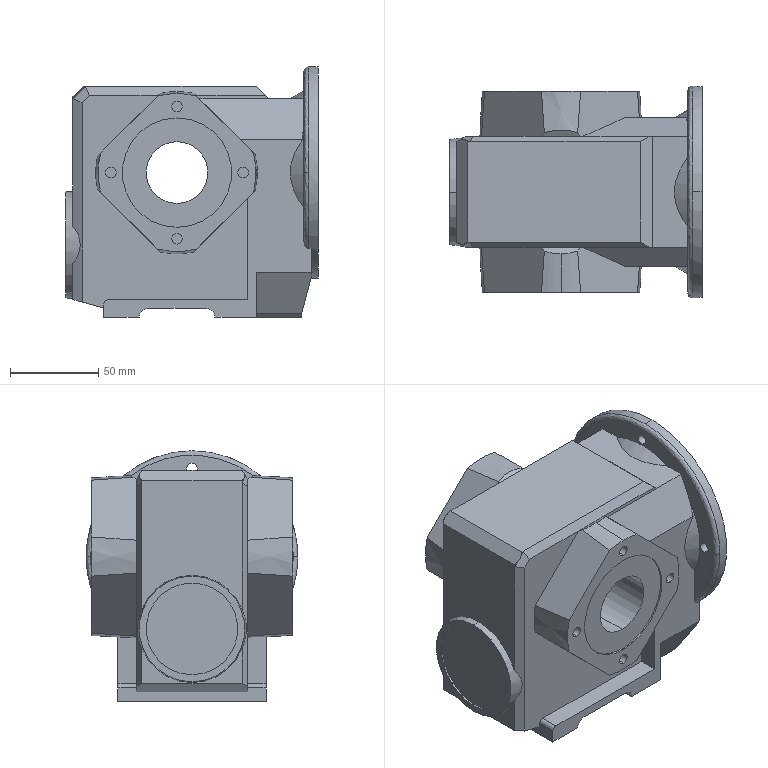Part | STEP file | PRODUCT_NAME_32_default | 1 solid | 133 faces | box 143 x 120 x 142 mm | volume 1389830 mm3 | plane 75 | cylinder 40 | cone 15 | spline 3 | commonest cylinder face diameters 6 x24 62 x4 5 x2 10 x2 35 x2 52 x2